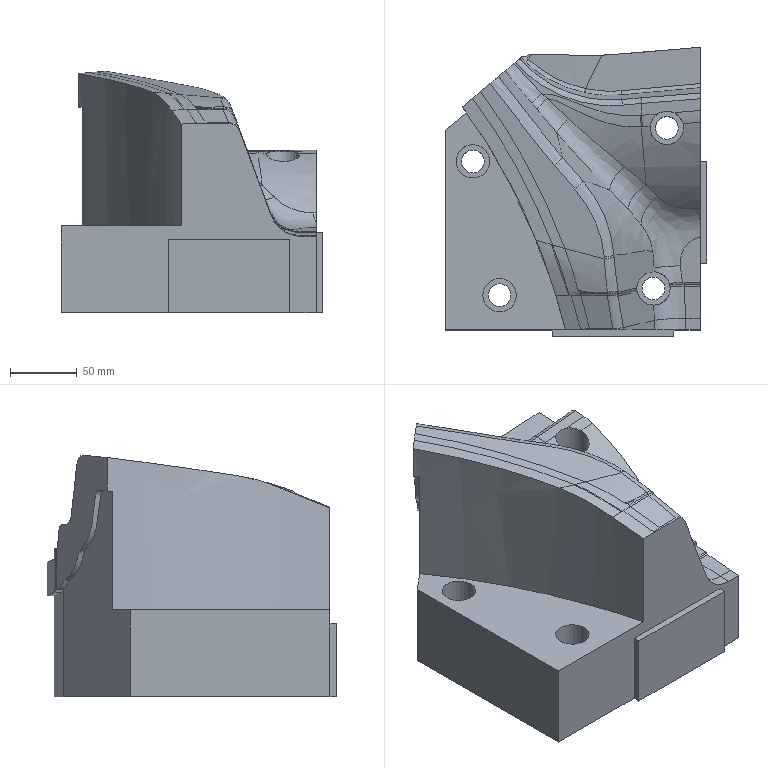Part | NX | features solid 2 | 1 solid | 111 faces | box 195.802 x 216.234 x 180.55 mm | volume 3962609 mm3 | spline 60 | plane 28 | cylinder 23 | commonest cylinder face diameters 6 x6 17 x4 25 x4 80 x2 6.022 x1 16 x1